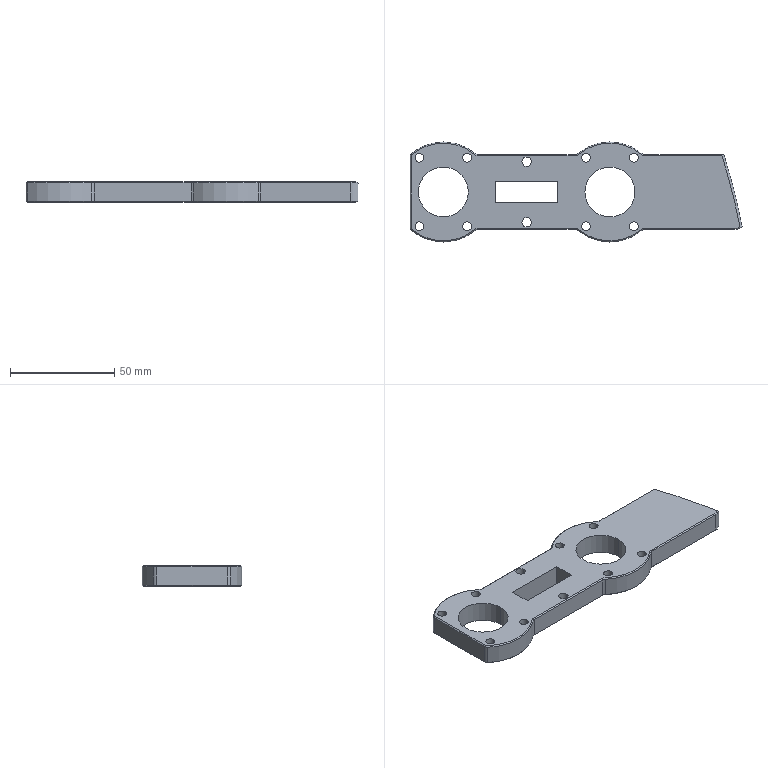Part | Creo | features DATUM PLANE 3, CHAMFER 2, CURVE 2, COORDINATE SYSTEM 1, CUT 1, PROTRUSION 1, ROUND 1 | 1 solid | 87 faces | volume 47470 mm3 | cylinder 38 | cone 28 | plane 21 | commonest cylinder face diameters 4.2 x16 4 x8 4.5 x4 24 x4 48 x4 10 x1